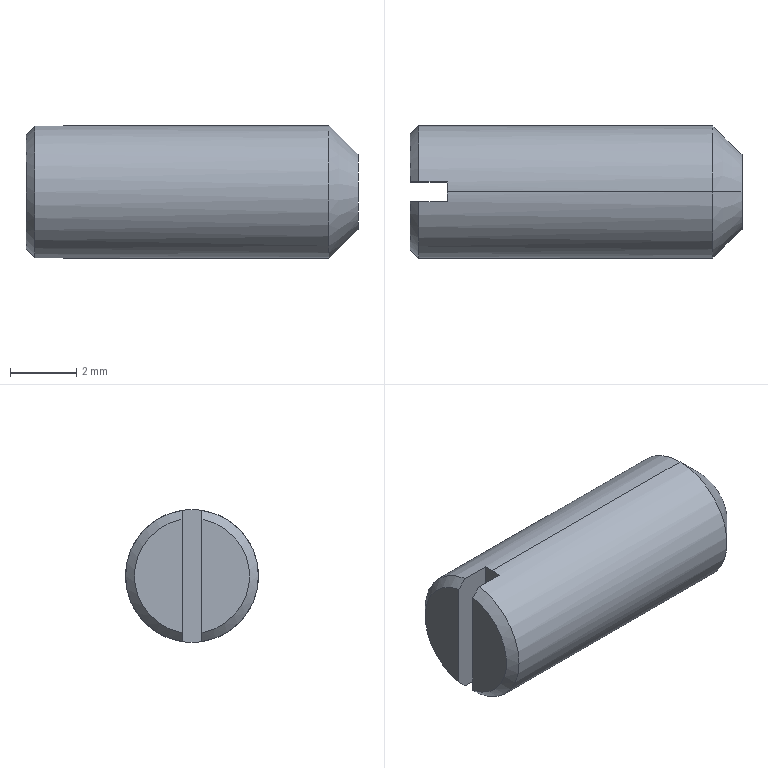Part | STEP file | 1 solid | 12 faces | box 10 x 4 x 4 mm | volume 118.489 mm3 | plane 6 | cone 4 | cylinder 2 | commonest cylinder face diameters 4 x2
STEP:
#1=CARTESIAN_POINT('',(0.,0.,0.));
#2=DIRECTION('',(0.,0.,1.));
#3=DIRECTION('',(1.,0.,0.));
#4=AXIS2_PLACEMENT_3D('',#1,#2,#3);
#5=CARTESIAN_POINT('',(1.12,-0.3,-1.977));
#6=VERTEX_POINT('',#5);
#7=CARTESIAN_POINT('',(1.12,0.,-2.));
#8=VERTEX_POINT('',#7);
#9=CARTESIAN_POINT('',(1.12,0.,0.));
#10=DIRECTION('',(1.,0.,0.));
#11=DIRECTION('',(0.,0.,1.));
#12=AXIS2_PLACEMENT_3D('',#9,#10,#11);
#13=CIRCLE('',#12,2.);
#14=CARTESIAN_POINT('',(1.12,-0.3,-50.));
#15=DIRECTION('',(1.,0.,0.));
#16=DIRECTION('',(0.,1.,0.));
#17=AXIS2_PLACEMENT_3D('',#14,#15,#16);
#18=PLANE('',#17);
#19=CARTESIAN_POINT('',(0.3,50.));
#20=DIRECTION('',(0.,1.));
#21=AXIS2_PLACEMENT_2D('',#19,#20);
#22=CIRCLE('',#21,2.);
#23=(GEOMETRIC_REPRESENTATION_CONTEXT(2)PARAMETRIC_REPRESENTATION_CONTEXT()REPRESENTATION_CONTEXT('',''));
#24=DEFINITIONAL_REPRESENTATION('',(#22),#23);
#25=PCURVE('',#18,#24);
#26=CARTESIAN_POINT('',(-0.5499,0.,0.));
#27=DIRECTION('',(-1.,0.,0.));
#28=DIRECTION('',(0.,0.,1.));
#29=AXIS2_PLACEMENT_3D('',#26,#27,#28);
#30=CYLINDRICAL_SURFACE('',#29,2.);
#31=CARTESIAN_POINT('',(6.283,-1.67));
#32=DIRECTION('',(-1.,0.));
#33=VECTOR('',#32,1.);
#34=LINE('',#31,#33);
#35=(GEOMETRIC_REPRESENTATION_CONTEXT(2)PARAMETRIC_REPRESENTATION_CONTEXT()REPRESENTATION_CONTEXT('',''));
#36=DEFINITIONAL_REPRESENTATION('',(#34),#35);
#37=PCURVE('',#30,#36);
#38=SURFACE_CURVE('',#13,(#25,#37),.PCURVE_S1.);
#39=EDGE_CURVE('',#6,#8,#38,.T.);
#40=ORIENTED_EDGE('',*,*,#39,.F.);
#41=CARTESIAN_POINT('',(1.12,-0.3,1.977));
#42=VERTEX_POINT('',#41);
#43=CARTESIAN_POINT('',(1.12,-0.3,-50.));
#44=DIRECTION('',(0.,0.,1.));
#45=VECTOR('',#44,1.);
#46=LINE('',#43,#45);
#47=CARTESIAN_POINT('',(0.,0.));
#48=DIRECTION('',(0.,1.));
#49=VECTOR('',#48,1.);
#50=LINE('',#47,#49);
#51=(GEOMETRIC_REPRESENTATION_CONTEXT(2)PARAMETRIC_REPRESENTATION_CONTEXT()REPRESENTATION_CONTEXT('',''));
#52=DEFINITIONAL_REPRESENTATION('',(#50),#51);
#53=PCURVE('',#18,#52);
#54=CARTESIAN_POINT('',(0.,-0.3,-50.));
#55=DIRECTION('',(0.,-1.,0.));
#56=DIRECTION('',(0.,0.,-1.));
#57=AXIS2_PLACEMENT_3D('',#54,#55,#56);
#58=PLANE('',#57);
#59=CARTESIAN_POINT('',(0.,1.12));
#60=DIRECTION('',(-1.,0.));
#61=VECTOR('',#60,1.);
#62=LINE('',#59,#61);
#63=(GEOMETRIC_REPRESENTATION_CONTEXT(2)PARAMETRIC_REPRESENTATION_CONTEXT()REPRESENTATION_CONTEXT('',''));
#64=DEFINITIONAL_REPRESENTATION('',(#62),#63);
#65=PCURVE('',#58,#64);
#66=SURFACE_CURVE('',#46,(#53,#65),.PCURVE_S1.);
#67=EDGE_CURVE('',#6,#42,#66,.T.);
#68=ORIENTED_EDGE('',*,*,#67,.T.);
#69=CARTESIAN_POINT('',(1.12,0.,2.));
#70=VERTEX_POINT('',#69);
#71=CARTESIAN_POINT('',(1.12,0.,0.));
#72=DIRECTION('',(1.,0.,0.));
#73=DIRECTION('',(0.,0.,1.));
#74=AXIS2_PLACEMENT_3D('',#71,#72,#73);
#75=CIRCLE('',#74,2.);
#76=CARTESIAN_POINT('',(0.3,50.));
#77=DIRECTION('',(0.,1.));
#78=AXIS2_PLACEMENT_2D('',#76,#77);
#79=CIRCLE('',#78,2.);
#80=(GEOMETRIC_REPRESENTATION_CONTEXT(2)PARAMETRIC_REPRESENTATION_CONTEXT()REPRESENTATION_CONTEXT('',''));
#81=DEFINITIONAL_REPRESENTATION('',(#79),#80);
#82=PCURVE('',#18,#81);
#83=CARTESIAN_POINT('',(6.283,-1.67));
#84=DIRECTION('',(-1.,0.));
#85=VECTOR('',#84,1.);
#86=LINE('',#83,#85);
#87=(GEOMETRIC_REPRESENTATION_CONTEXT(2)PARAMETRIC_REPRESENTATION_CONTEXT()REPRESENTATION_CONTEXT('',''));
#88=DEFINITIONAL_REPRESENTATION('',(#86),#87);
#89=PCURVE('',#30,#88);
#90=SURFACE_CURVE('',#75,(#82,#89),.PCURVE_S1.);
#91=EDGE_CURVE('',#70,#42,#90,.T.);
#92=ORIENTED_EDGE('',*,*,#91,.F.);
#93=CARTESIAN_POINT('',(1.12,0.3,1.977));
#94=VERTEX_POINT('',#93);
#95=CARTESIAN_POINT('',(1.12,0.,0.));
#96=DIRECTION('',(1.,0.,0.));
#97=DIRECTION('',(0.,0.,1.));
#98=AXIS2_PLACEMENT_3D('',#95,#96,#97);
#99=CIRCLE('',#98,2.);
#100=CARTESIAN_POINT('',(0.3,50.));
#101=DIRECTION('',(0.,1.));
#102=AXIS2_PLACEMENT_2D('',#100,#101);
#103=CIRCLE('',#102,2.);
#104=(GEOMETRIC_REPRESENTATION_CONTEXT(2)PARAMETRIC_REPRESENTATION_CONTEXT()REPRESENTATION_CONTEXT('',''));
#105=DEFINITIONAL_REPRESENTATION('',(#103),#104);
#106=PCURVE('',#18,#105);
#107=CARTESIAN_POINT('',(-0.5499,0.,0.));
#108=DIRECTION('',(-1.,0.,0.));
#109=DIRECTION('',(0.,0.,1.));
#110=AXIS2_PLACEMENT_3D('',#107,#108,#109);
#111=CYLINDRICAL_SURFACE('',#110,2.);
#112=CARTESIAN_POINT('',(6.283,-1.67));
#113=DIRECTION('',(-1.,0.));
#114=VECTOR('',#113,1.);
#115=LINE('',#112,#114);
#116=(GEOMETRIC_REPRESENTATION_CONTEXT(2)PARAMETRIC_REPRESENTATION_CONTEXT()REPRESENTATION_CONTEXT('',''));
#117=DEFINITIONAL_REPRESENTATION('',(#115),#116);
#118=PCURVE('',#111,#117);
#119=SURFACE_CURVE('',#99,(#106,#118),.PCURVE_S1.);
#120=EDGE_CURVE('',#94,#70,#119,.T.);
#121=ORIENTED_EDGE('',*,*,#120,.F.);
#122=CARTESIAN_POINT('',(1.12,0.3,-1.977));
#123=VERTEX_POINT('',#122);
#124=CARTESIAN_POINT('',(1.12,0.3,-50.));
#125=DIRECTION('',(0.,0.,-1.));
#126=VECTOR('',#125,1.);
#127=LINE('',#124,#126);
#128=CARTESIAN_POINT('',(0.6,0.));
#129=DIRECTION('',(0.,-1.));
#130=VECTOR('',#129,1.);
#131=LINE('',#128,#130);
#132=(GEOMETRIC_REPRESENTATION_CONTEXT(2)PARAMETRIC_REPRESENTATION_CONTEXT()REPRESENTATION_CONTEXT('',''));
#133=DEFINITIONAL_REPRESENTATION('',(#131),#132);
#134=PCURVE('',#18,#133);
#135=CARTESIAN_POINT('',(0.,0.3,-50.));
#136=DIRECTION('',(0.,1.,0.));
#137=DIRECTION('',(1.,0.,0.));
#138=AXIS2_PLACEMENT_3D('',#135,#136,#137);
#139=PLANE('',#138);
#140=CARTESIAN_POINT('',(1.12,0.));
#141=DIRECTION('',(0.,1.));
#142=VECTOR('',#141,1.);
#143=LINE('',#140,#142);
#144=(GEOMETRIC_REPRESENTATION_CONTEXT(2)PARAMETRIC_REPRESENTATION_CONTEXT()REPRESENTATION_CONTEXT('',''));
#145=DEFINITIONAL_REPRESENTATION('',(#143),#144);
#146=PCURVE('',#139,#145);
#147=SURFACE_CURVE('',#127,(#134,#146),.PCURVE_S1.);
#148=EDGE_CURVE('',#94,#123,#147,.T.);
#149=ORIENTED_EDGE('',*,*,#148,.T.);
#150=CARTESIAN_POINT('',(1.12,0.,0.));
#151=DIRECTION('',(1.,0.,0.));
#152=DIRECTION('',(0.,0.,1.));
#153=AXIS2_PLACEMENT_3D('',#150,#151,#152);
#154=CIRCLE('',#153,2.);
#155=CARTESIAN_POINT('',(0.3,50.));
#156=DIRECTION('',(0.,1.));
#157=AXIS2_PLACEMENT_2D('',#155,#156);
#158=CIRCLE('',#157,2.);
#159=(GEOMETRIC_REPRESENTATION_CONTEXT(2)PARAMETRIC_REPRESENTATION_CONTEXT()REPRESENTATION_CONTEXT('',''));
#160=DEFINITIONAL_REPRESENTATION('',(#158),#159);
#161=PCURVE('',#18,#160);
#162=CARTESIAN_POINT('',(6.283,-1.67));
#163=DIRECTION('',(-1.,0.));
#164=VECTOR('',#163,1.);
#165=LINE('',#162,#164);
#166=(GEOMETRIC_REPRESENTATION_CONTEXT(2)PARAMETRIC_REPRESENTATION_CONTEXT()REPRESENTATION_CONTEXT('',''));
#167=DEFINITIONAL_REPRESENTATION('',(#165),#166);
#168=PCURVE('',#111,#167);
#169=SURFACE_CURVE('',#154,(#161,#168),.PCURVE_S1.);
#170=EDGE_CURVE('',#8,#123,#169,.T.);
#171=ORIENTED_EDGE('',*,*,#170,.F.);
#172=EDGE_LOOP('',(#40,#68,#92,#121,#149,#171));
#173=FACE_BOUND('',#172,.T.);
#174=ADVANCED_FACE('',(#173),#18,.F.);
#175=CARTESIAN_POINT('',(0.268,-0.3,-1.977));
#176=VERTEX_POINT('',#175);
#177=CARTESIAN_POINT('',(0.,-0.3,-1.977));
#178=DIRECTION('',(1.,0.,0.));
#179=VECTOR('',#178,1.);
#180=LINE('',#177,#179);
#181=CARTESIAN_POINT('',(-48.023,0.));
#182=DIRECTION('',(0.,1.));
#183=VECTOR('',#182,1.);
#184=LINE('',#181,#183);
#185=(GEOMETRIC_REPRESENTATION_CONTEXT(2)PARAMETRIC_REPRESENTATION_CONTEXT()REPRESENTATION_CONTEXT('',''));
#186=DEFINITIONAL_REPRESENTATION('',(#184),#185);
#187=PCURVE('',#58,#186);
#188=CARTESIAN_POINT('',(3.292,-0.5499));
#189=DIRECTION('',(0.,-1.));
#190=VECTOR('',#189,1.);
#191=LINE('',#188,#190);
#192=(GEOMETRIC_REPRESENTATION_CONTEXT(2)PARAMETRIC_REPRESENTATION_CONTEXT()REPRESENTATION_CONTEXT('',''));
#193=DEFINITIONAL_REPRESENTATION('',(#191),#192);
#194=PCURVE('',#30,#193);
#195=SURFACE_CURVE('',#180,(#187,#194),.PCURVE_S1.);
#196=EDGE_CURVE('',#176,#6,#195,.T.);
#197=ORIENTED_EDGE('',*,*,#196,.F.);
#198=CARTESIAN_POINT('',(0.,-0.3,-1.706));
#199=VERTEX_POINT('',#198);
#200=CARTESIAN_POINT('',(0.,-0.3,-1.706));
#201=CARTESIAN_POINT('',(0.08924,-0.3,-1.796));
#202=CARTESIAN_POINT('',(0.1786,-0.3,-1.887));
#203=CARTESIAN_POINT('',(0.268,-0.3,-1.977));
#204=B_SPLINE_CURVE_WITH_KNOTS('',3,(#200,#201,#202,#203),.UNSPECIFIED.,.F.,.F.,(4,4),(0.,0.0003815),.PIECEWISE_BEZIER_KNOTS.);
#205=CARTESIAN_POINT('',(-48.294,0.));
#206=CARTESIAN_POINT('',(-48.204,0.08924));
#207=CARTESIAN_POINT('',(-48.113,0.1786));
#208=CARTESIAN_POINT('',(-48.023,0.268));
#209=B_SPLINE_CURVE_WITH_KNOTS('',3,(#205,#206,#207,#208),.UNSPECIFIED.,.F.,.F.,(4,4),(0.,0.0003815),.PIECEWISE_BEZIER_KNOTS.);
#210=(GEOMETRIC_REPRESENTATION_CONTEXT(2)PARAMETRIC_REPRESENTATION_CONTEXT()REPRESENTATION_CONTEXT('',''));
#211=DEFINITIONAL_REPRESENTATION('',(#209),#210);
#212=PCURVE('',#58,#211);
#213=CARTESIAN_POINT('',(0.268,0.,0.));
#214=DIRECTION('',(1.,0.,0.));
#215=DIRECTION('',(0.,0.,-1.));
#216=AXIS2_PLACEMENT_3D('',#213,#214,#215);
#217=CONICAL_SURFACE('',#216,2.,0.7854);
#218=CARTESIAN_POINT('',(6.109,-0.268));
#219=CARTESIAN_POINT('',(6.11,-0.2639));
#220=CARTESIAN_POINT('',(6.11,-0.2558));
#221=CARTESIAN_POINT('',(6.112,-0.2437));
#222=CARTESIAN_POINT('',(6.113,-0.2315));
#223=CARTESIAN_POINT('',(6.114,-0.2193));
#224=CARTESIAN_POINT('',(6.115,-0.2071));
#225=CARTESIAN_POINT('',(6.116,-0.195));
#226=CARTESIAN_POINT('',(6.117,-0.1828));
#227=CARTESIAN_POINT('',(6.118,-0.1706));
#228=CARTESIAN_POINT('',(6.12,-0.1584));
#229=CARTESIAN_POINT('',(6.121,-0.1462));
#230=CARTESIAN_POINT('',(6.122,-0.1341));
#231=CARTESIAN_POINT('',(6.123,-0.1219));
#232=CARTESIAN_POINT('',(6.124,-0.1097));
#233=CARTESIAN_POINT('',(6.125,-0.09751));
#234=CARTESIAN_POINT('',(6.126,-0.08533));
#235=CARTESIAN_POINT('',(6.127,-0.07314));
#236=CARTESIAN_POINT('',(6.128,-0.06095));
#237=CARTESIAN_POINT('',(6.129,-0.04876));
#238=CARTESIAN_POINT('',(6.13,-0.03657));
#239=CARTESIAN_POINT('',(6.131,-0.02438));
#240=CARTESIAN_POINT('',(6.132,-0.01219));
#241=CARTESIAN_POINT('',(6.132,-0.004064));
#242=CARTESIAN_POINT('',(6.133,0.));
#243=B_SPLINE_CURVE_WITH_KNOTS('',3,(#218,#219,#220,#221,#222,#223,#224,#225,#226,#227,#228,#229,#230,#231,#232,#233,#234,#235,#236,#237,#238,#239,#240,#241,#242),.UNSPECIFIED.,.F.,.F.,(4,1,1,1,1,1,1,1,1,1,1,1,1,1,1,1,1,1,1,1,1,1,4),(0.,0.00001734,0.00003468,0.00005203,0.00006937,0.00008671,0.0001041,0.0001214,0.0001387,0.0001561,0.0001734,0.0001908,0.0002081,0.0002254,0.0002428,0.0002601,0.0002775,0.0002948,0.0003122,0.0003295,0.0003468,0.0003642,0.0003815),.QUASI_UNIFORM_KNOTS.);
#244=(GEOMETRIC_REPRESENTATION_CONTEXT(2)PARAMETRIC_REPRESENTATION_CONTEXT()REPRESENTATION_CONTEXT('',''));
#245=DEFINITIONAL_REPRESENTATION('',(#243),#244);
#246=PCURVE('',#217,#245);
#247=SURFACE_CURVE('',#204,(#212,#246),.PCURVE_S1.);
#248=EDGE_CURVE('',#199,#176,#247,.T.);
#249=ORIENTED_EDGE('',*,*,#248,.F.);
#250=CARTESIAN_POINT('',(0.,-0.3,1.706));
#251=VERTEX_POINT('',#250);
#252=CARTESIAN_POINT('',(0.,-0.3,0.));
#253=DIRECTION('',(0.,0.,1.));
#254=VECTOR('',#253,1.);
#255=LINE('',#252,#254);
#256=CARTESIAN_POINT('',(-50.,0.));
#257=DIRECTION('',(-1.,0.));
#258=VECTOR('',#257,1.);
#259=LINE('',#256,#258);
#260=(GEOMETRIC_REPRESENTATION_CONTEXT(2)PARAMETRIC_REPRESENTATION_CONTEXT()REPRESENTATION_CONTEXT('',''));
#261=DEFINITIONAL_REPRESENTATION('',(#259),#260);
#262=PCURVE('',#58,#261);
#263=CARTESIAN_POINT('',(0.,1.732,0.));
#264=DIRECTION('',(1.,0.,0.));
#265=DIRECTION('',(0.,1.,0.));
#266=AXIS2_PLACEMENT_3D('',#263,#264,#265);
#267=PLANE('',#266);
#268=CARTESIAN_POINT('',(-2.032,0.));
#269=DIRECTION('',(0.,1.));
#270=VECTOR('',#269,1.);
#271=LINE('',#268,#270);
#272=(GEOMETRIC_REPRESENTATION_CONTEXT(2)PARAMETRIC_REPRESENTATION_CONTEXT()REPRESENTATION_CONTEXT('',''));
#273=DEFINITIONAL_REPRESENTATION('',(#271),#272);
#274=PCURVE('',#267,#273);
#275=SURFACE_CURVE('',#255,(#262,#274),.PCURVE_S1.);
#276=EDGE_CURVE('',#199,#251,#275,.T.);
#277=ORIENTED_EDGE('',*,*,#276,.T.);
#278=CARTESIAN_POINT('',(0.268,-0.3,1.977));
#279=VERTEX_POINT('',#278);
#280=CARTESIAN_POINT('',(0.268,-0.3,1.977));
#281=CARTESIAN_POINT('',(0.1786,-0.3,1.887));
#282=CARTESIAN_POINT('',(0.08924,-0.3,1.796));
#283=CARTESIAN_POINT('',(0.,-0.3,1.706));
#284=B_SPLINE_CURVE_WITH_KNOTS('',3,(#280,#281,#282,#283),.UNSPECIFIED.,.F.,.F.,(4,4),(0.,0.0003815),.PIECEWISE_BEZIER_KNOTS.);
#285=CARTESIAN_POINT('',(-51.977,0.268));
#286=CARTESIAN_POINT('',(-51.887,0.1786));
#287=CARTESIAN_POINT('',(-51.796,0.08924));
#288=CARTESIAN_POINT('',(-51.706,0.));
#289=B_SPLINE_CURVE_WITH_KNOTS('',3,(#285,#286,#287,#288),.UNSPECIFIED.,.F.,.F.,(4,4),(0.,0.0003815),.PIECEWISE_BEZIER_KNOTS.);
#290=(GEOMETRIC_REPRESENTATION_CONTEXT(2)PARAMETRIC_REPRESENTATION_CONTEXT()REPRESENTATION_CONTEXT('',''));
#291=DEFINITIONAL_REPRESENTATION('',(#289),#290);
#292=PCURVE('',#58,#291);
#293=CARTESIAN_POINT('',(3.292,0.));
#294=CARTESIAN_POINT('',(3.292,-0.004064));
#295=CARTESIAN_POINT('',(3.293,-0.01219));
#296=CARTESIAN_POINT('',(3.294,-0.02438));
#297=CARTESIAN_POINT('',(3.295,-0.03657));
#298=CARTESIAN_POINT('',(3.296,-0.04876));
#299=CARTESIAN_POINT('',(3.297,-0.06095));
#300=CARTESIAN_POINT('',(3.298,-0.07314));
#301=CARTESIAN_POINT('',(3.299,-0.08533));
#302=CARTESIAN_POINT('',(3.3,-0.09751));
#303=CARTESIAN_POINT('',(3.301,-0.1097));
#304=CARTESIAN_POINT('',(3.302,-0.1219));
#305=CARTESIAN_POINT('',(3.303,-0.1341));
#306=CARTESIAN_POINT('',(3.304,-0.1462));
#307=CARTESIAN_POINT('',(3.305,-0.1584));
#308=CARTESIAN_POINT('',(3.306,-0.1706));
#309=CARTESIAN_POINT('',(3.307,-0.1828));
#310=CARTESIAN_POINT('',(3.309,-0.195));
#311=CARTESIAN_POINT('',(3.31,-0.2071));
#312=CARTESIAN_POINT('',(3.311,-0.2193));
#313=CARTESIAN_POINT('',(3.312,-0.2315));
#314=CARTESIAN_POINT('',(3.313,-0.2437));
#315=CARTESIAN_POINT('',(3.314,-0.2558));
#316=CARTESIAN_POINT('',(3.315,-0.2639));
#317=CARTESIAN_POINT('',(3.316,-0.268));
#318=B_SPLINE_CURVE_WITH_KNOTS('',3,(#293,#294,#295,#296,#297,#298,#299,#300,#301,#302,#303,#304,#305,#306,#307,#308,#309,#310,#311,#312,#313,#314,#315,#316,#317),.UNSPECIFIED.,.F.,.F.,(4,1,1,1,1,1,1,1,1,1,1,1,1,1,1,1,1,1,1,1,1,1,4),(0.,0.00001734,0.00003468,0.00005203,0.00006937,0.00008671,0.0001041,0.0001214,0.0001387,0.0001561,0.0001734,0.0001908,0.0002081,0.0002254,0.0002428,0.0002601,0.0002775,0.0002948,0.0003122,0.0003295,0.0003468,0.0003642,0.0003815),.QUASI_UNIFORM_KNOTS.);
#319=(GEOMETRIC_REPRESENTATION_CONTEXT(2)PARAMETRIC_REPRESENTATION_CONTEXT()REPRESENTATION_CONTEXT('',''));
#320=DEFINITIONAL_REPRESENTATION('',(#318),#319);
#321=PCURVE('',#217,#320);
#322=SURFACE_CURVE('',#284,(#292,#321),.PCURVE_S1.);
#323=EDGE_CURVE('',#279,#251,#322,.T.);
#324=ORIENTED_EDGE('',*,*,#323,.F.);
#325=CARTESIAN_POINT('',(0.,-0.3,1.977));
#326=DIRECTION('',(-1.,0.,0.));
#327=VECTOR('',#326,1.);
#328=LINE('',#325,#327);
#329=CARTESIAN_POINT('',(-51.977,0.));
#330=DIRECTION('',(0.,-1.));
#331=VECTOR('',#330,1.);
#332=LINE('',#329,#331);
#333=(GEOMETRIC_REPRESENTATION_CONTEXT(2)PARAMETRIC_REPRESENTATION_CONTEXT()REPRESENTATION_CONTEXT('',''));
#334=DEFINITIONAL_REPRESENTATION('',(#332),#333);
#335=PCURVE('',#58,#334);
#336=CARTESIAN_POINT('',(6.133,-0.5499));
#337=DIRECTION('',(0.,1.));
#338=VECTOR('',#337,1.);
#339=LINE('',#336,#338);
#340=(GEOMETRIC_REPRESENTATION_CONTEXT(2)PARAMETRIC_REPRESENTATION_CONTEXT()REPRESENTATION_CONTEXT('',''));
#341=DEFINITIONAL_REPRESENTATION('',(#339),#340);
#342=PCURVE('',#30,#341);
#343=SURFACE_CURVE('',#328,(#335,#342),.PCURVE_S1.);
#344=EDGE_CURVE('',#42,#279,#343,.T.);
#345=ORIENTED_EDGE('',*,*,#344,.F.);
#346=ORIENTED_EDGE('',*,*,#67,.F.);
#347=EDGE_LOOP('',(#197,#249,#277,#324,#345,#346));
#348=FACE_BOUND('',#347,.T.);
#349=ADVANCED_FACE('',(#348),#58,.F.);
#350=CARTESIAN_POINT('',(0.268,0.3,1.977));
#351=VERTEX_POINT('',#350);
#352=CARTESIAN_POINT('',(0.,0.3,1.977));
#353=DIRECTION('',(1.,0.,0.));
#354=VECTOR('',#353,1.);
#355=LINE('',#352,#354);
#356=CARTESIAN_POINT('',(0.,-51.977));
#357=DIRECTION('',(1.,0.));
#358=VECTOR('',#357,1.);
#359=LINE('',#356,#358);
#360=(GEOMETRIC_REPRESENTATION_CONTEXT(2)PARAMETRIC_REPRESENTATION_CONTEXT()REPRESENTATION_CONTEXT('',''));
#361=DEFINITIONAL_REPRESENTATION('',(#359),#360);
#362=PCURVE('',#139,#361);
#363=CARTESIAN_POINT('',(0.1506,-0.5499));
#364=DIRECTION('',(0.,-1.));
#365=VECTOR('',#364,1.);
#366=LINE('',#363,#365);
#367=(GEOMETRIC_REPRESENTATION_CONTEXT(2)PARAMETRIC_REPRESENTATION_CONTEXT()REPRESENTATION_CONTEXT('',''));
#368=DEFINITIONAL_REPRESENTATION('',(#366),#367);
#369=PCURVE('',#111,#368);
#370=SURFACE_CURVE('',#355,(#362,#369),.PCURVE_S1.);
#371=EDGE_CURVE('',#351,#94,#370,.T.);
#372=ORIENTED_EDGE('',*,*,#371,.F.);
#373=CARTESIAN_POINT('',(0.,0.3,1.706));
#374=VERTEX_POINT('',#373);
#375=CARTESIAN_POINT('',(0.,0.3,1.706));
#376=CARTESIAN_POINT('',(0.08924,0.3,1.796));
#377=CARTESIAN_POINT('',(0.1786,0.3,1.887));
#378=CARTESIAN_POINT('',(0.268,0.3,1.977));
#379=B_SPLINE_CURVE_WITH_KNOTS('',3,(#375,#376,#377,#378),.UNSPECIFIED.,.F.,.F.,(4,4),(0.,0.0003815),.PIECEWISE_BEZIER_KNOTS.);
#380=CARTESIAN_POINT('',(0.,-51.706));
#381=CARTESIAN_POINT('',(0.08924,-51.796));
#382=CARTESIAN_POINT('',(0.1786,-51.887));
#383=CARTESIAN_POINT('',(0.268,-51.977));
#384=B_SPLINE_CURVE_WITH_KNOTS('',3,(#380,#381,#382,#383),.UNSPECIFIED.,.F.,.F.,(4,4),(0.,0.0003815),.PIECEWISE_BEZIER_KNOTS.);
#385=(GEOMETRIC_REPRESENTATION_CONTEXT(2)PARAMETRIC_REPRESENTATION_CONTEXT()REPRESENTATION_CONTEXT('',''));
#386=DEFINITIONAL_REPRESENTATION('',(#384),#385);
#387=PCURVE('',#139,#386);
#388=CARTESIAN_POINT('',(0.268,0.,0.));
#389=DIRECTION('',(1.,0.,0.));
#390=DIRECTION('',(0.,0.,-1.));
#391=AXIS2_PLACEMENT_3D('',#388,#389,#390);
#392=CONICAL_SURFACE('',#391,2.,0.7854);
#393=CARTESIAN_POINT('',(2.968,-0.268));
#394=CARTESIAN_POINT('',(2.968,-0.2639));
#395=CARTESIAN_POINT('',(2.969,-0.2558));
#396=CARTESIAN_POINT('',(2.97,-0.2437));
#397=CARTESIAN_POINT('',(2.971,-0.2315));
#398=CARTESIAN_POINT('',(2.972,-0.2193));
#399=CARTESIAN_POINT('',(2.973,-0.2071));
#400=CARTESIAN_POINT('',(2.975,-0.195));
#401=CARTESIAN_POINT('',(2.976,-0.1828));
#402=CARTESIAN_POINT('',(2.977,-0.1706));
#403=CARTESIAN_POINT('',(2.978,-0.1584));
#404=CARTESIAN_POINT('',(2.979,-0.1462));
#405=CARTESIAN_POINT('',(2.98,-0.1341));
#406=CARTESIAN_POINT('',(2.981,-0.1219));
#407=CARTESIAN_POINT('',(2.982,-0.1097));
#408=CARTESIAN_POINT('',(2.983,-0.09751));
#409=CARTESIAN_POINT('',(2.984,-0.08533));
#410=CARTESIAN_POINT('',(2.985,-0.07314));
#411=CARTESIAN_POINT('',(2.986,-0.06095));
#412=CARTESIAN_POINT('',(2.987,-0.04876));
#413=CARTESIAN_POINT('',(2.988,-0.03657));
#414=CARTESIAN_POINT('',(2.989,-0.02438));
#415=CARTESIAN_POINT('',(2.99,-0.01219));
#416=CARTESIAN_POINT('',(2.991,-0.004064));
#417=CARTESIAN_POINT('',(2.991,0.));
#418=B_SPLINE_CURVE_WITH_KNOTS('',3,(#393,#394,#395,#396,#397,#398,#399,#400,#401,#402,#403,#404,#405,#406,#407,#408,#409,#410,#411,#412,#413,#414,#415,#416,#417),.UNSPECIFIED.,.F.,.F.,(4,1,1,1,1,1,1,1,1,1,1,1,1,1,1,1,1,1,1,1,1,1,4),(0.,0.00001734,0.00003468,0.00005203,0.00006937,0.00008671,0.0001041,0.0001214,0.0001387,0.0001561,0.0001734,0.0001908,0.0002081,0.0002254,0.0002428,0.0002601,0.0002775,0.0002948,0.0003122,0.0003295,0.0003468,0.0003642,0.0003815),.QUASI_UNIFORM_KNOTS.);
#419=(GEOMETRIC_REPRESENTATION_CONTEXT(2)PARAMETRIC_REPRESENTATION_CONTEXT()REPRESENTATION_CONTEXT('',''));
#420=DEFINITIONAL_REPRESENTATION('',(#418),#419);
#421=PCURVE('',#392,#420);
#422=SURFACE_CURVE('',#379,(#387,#421),.PCURVE_S1.);
#423=EDGE_CURVE('',#374,#351,#422,.T.);
#424=ORIENTED_EDGE('',*,*,#423,.F.);
#425=CARTESIAN_POINT('',(0.,0.3,-1.706));
#426=VERTEX_POINT('',#425);
#427=CARTESIAN_POINT('',(0.,0.3,0.));
#428=DIRECTION('',(0.,0.,-1.));
#429=VECTOR('',#428,1.);
#430=LINE('',#427,#429);
#431=CARTESIAN_POINT('',(0.,-50.));
#432=DIRECTION('',(0.,1.));
#433=VECTOR('',#432,1.);
#434=LINE('',#431,#433);
#435=(GEOMETRIC_REPRESENTATION_CONTEXT(2)PARAMETRIC_REPRESENTATION_CONTEXT()REPRESENTATION_CONTEXT('',''));
#436=DEFINITIONAL_REPRESENTATION('',(#434),#435);
#437=PCURVE('',#139,#436);
#438=CARTESIAN_POINT('',(0.,1.732,0.));
#439=DIRECTION('',(1.,0.,0.));
#440=DIRECTION('',(0.,1.,0.));
#441=AXIS2_PLACEMENT_3D('',#438,#439,#440);
#442=PLANE('',#441);
#443=CARTESIAN_POINT('',(-1.432,0.));
#444=DIRECTION('',(0.,-1.));
#445=VECTOR('',#444,1.);
#446=LINE('',#443,#445);
#447=(GEOMETRIC_REPRESENTATION_CONTEXT(2)PARAMETRIC_REPRESENTATION_CONTEXT()REPRESENTATION_CONTEXT('',''));
#448=DEFINITIONAL_REPRESENTATION('',(#446),#447);
#449=PCURVE('',#442,#448);
#450=SURFACE_CURVE('',#430,(#437,#449),.PCURVE_S1.);
#451=EDGE_CURVE('',#374,#426,#450,.T.);
#452=ORIENTED_EDGE('',*,*,#451,.T.);
#453=CARTESIAN_POINT('',(0.268,0.3,-1.977));
#454=VERTEX_POINT('',#453);
#455=CARTESIAN_POINT('',(0.268,0.3,-1.977));
#456=CARTESIAN_POINT('',(0.1786,0.3,-1.887));
#457=CARTESIAN_POINT('',(0.08924,0.3,-1.796));
#458=CARTESIAN_POINT('',(0.,0.3,-1.706));
#459=B_SPLINE_CURVE_WITH_KNOTS('',3,(#455,#456,#457,#458),.UNSPECIFIED.,.F.,.F.,(4,4),(0.,0.0003815),.PIECEWISE_BEZIER_KNOTS.);
#460=CARTESIAN_POINT('',(0.268,-48.023));
#461=CARTESIAN_POINT('',(0.1786,-48.113));
#462=CARTESIAN_POINT('',(0.08924,-48.204));
#463=CARTESIAN_POINT('',(0.,-48.294));
#464=B_SPLINE_CURVE_WITH_KNOTS('',3,(#460,#461,#462,#463),.UNSPECIFIED.,.F.,.F.,(4,4),(0.,0.0003815),.PIECEWISE_BEZIER_KNOTS.);
#465=(GEOMETRIC_REPRESENTATION_CONTEXT(2)PARAMETRIC_REPRESENTATION_CONTEXT()REPRESENTATION_CONTEXT('',''));
#466=DEFINITIONAL_REPRESENTATION('',(#464),#465);
#467=PCURVE('',#139,#466);
#468=CARTESIAN_POINT('',(0.1506,0.));
#469=CARTESIAN_POINT('',(0.1509,-0.004064));
#470=CARTESIAN_POINT('',(0.1515,-0.01219));
#471=CARTESIAN_POINT('',(0.1524,-0.02438));
#472=CARTESIAN_POINT('',(0.1534,-0.03657));
#473=CARTESIAN_POINT('',(0.1544,-0.04876));
#474=CARTESIAN_POINT('',(0.1553,-0.06095));
#475=CARTESIAN_POINT('',(0.1563,-0.07314));
#476=CARTESIAN_POINT('',(0.1573,-0.08533));
#477=CARTESIAN_POINT('',(0.1583,-0.09751));
#478=CARTESIAN_POINT('',(0.1594,-0.1097));
#479=CARTESIAN_POINT('',(0.1604,-0.1219));
#480=CARTESIAN_POINT('',(0.1615,-0.1341));
#481=CARTESIAN_POINT('',(0.1625,-0.1462));
#482=CARTESIAN_POINT('',(0.1636,-0.1584));
#483=CARTESIAN_POINT('',(0.1647,-0.1706));
#484=CARTESIAN_POINT('',(0.1658,-0.1828));
#485=CARTESIAN_POINT('',(0.167,-0.195));
#486=CARTESIAN_POINT('',(0.1681,-0.2071));
#487=CARTESIAN_POINT('',(0.1693,-0.2193));
#488=CARTESIAN_POINT('',(0.1705,-0.2315));
#489=CARTESIAN_POINT('',(0.1716,-0.2437));
#490=CARTESIAN_POINT('',(0.1729,-0.2558));
#491=CARTESIAN_POINT('',(0.1737,-0.2639));
#492=CARTESIAN_POINT('',(0.1741,-0.268));
#493=B_SPLINE_CURVE_WITH_KNOTS('',3,(#468,#469,#470,#471,#472,#473,#474,#475,#476,#477,#478,#479,#480,#481,#482,#483,#484,#485,#486,#487,#488,#489,#490,#491,#492),.UNSPECIFIED.,.F.,.F.,(4,1,1,1,1,1,1,1,1,1,1,1,1,1,1,1,1,1,1,1,1,1,4),(0.,0.00001734,0.00003468,0.00005203,0.00006937,0.00008671,0.0001041,0.0001214,0.0001387,0.0001561,0.0001734,0.0001908,0.0002081,0.0002254,0.0002428,0.0002601,0.0002775,0.0002948,0.0003122,0.0003295,0.0003468,0.0003642,0.0003815),.QUASI_UNIFORM_KNOTS.);
#494=(GEOMETRIC_REPRESENTATION_CONTEXT(2)PARAMETRIC_REPRESENTATION_CONTEXT()REPRESENTATION_CONTEXT('',''));
#495=DEFINITIONAL_REPRESENTATION('',(#493),#494);
#496=PCURVE('',#392,#495);
#497=SURFACE_CURVE('',#459,(#467,#496),.PCURVE_S1.);
#498=EDGE_CURVE('',#454,#426,#497,.T.);
#499=ORIENTED_EDGE('',*,*,#498,.F.);
#500=CARTESIAN_POINT('',(0.,0.3,-1.977));
#501=DIRECTION('',(-1.,0.,0.));
#502=VECTOR('',#501,1.);
#503=LINE('',#500,#502);
#504=CARTESIAN_POINT('',(0.,-48.023));
#505=DIRECTION('',(-1.,0.));
#506=VECTOR('',#505,1.);
#507=LINE('',#504,#506);
#508=(GEOMETRIC_REPRESENTATION_CONTEXT(2)PARAMETRIC_REPRESENTATION_CONTEXT()REPRESENTATION_CONTEXT('',''));
#509=DEFINITIONAL_REPRESENTATION('',(#507),#508);
#510=PCURVE('',#139,#509);
#511=CARTESIAN_POINT('',(2.991,-0.5499));
#512=DIRECTION('',(0.,1.));
#513=VECTOR('',#512,1.);
#514=LINE('',#511,#513);
#515=(GEOMETRIC_REPRESENTATION_CONTEXT(2)PARAMETRIC_REPRESENTATION_CONTEXT()REPRESENTATION_CONTEXT('',''));
#516=DEFINITIONAL_REPRESENTATION('',(#514),#515);
#517=PCURVE('',#111,#516);
#518=SURFACE_CURVE('',#503,(#510,#517),.PCURVE_S1.);
#519=EDGE_CURVE('',#123,#454,#518,.T.);
#520=ORIENTED_EDGE('',*,*,#519,.F.);
#521=ORIENTED_EDGE('',*,*,#148,.F.);
#522=EDGE_LOOP('',(#372,#424,#452,#499,#520,#521));
#523=FACE_BOUND('',#522,.T.);
#524=ADVANCED_FACE('',(#523),#139,.F.);
#525=ORIENTED_EDGE('',*,*,#276,.F.);
#526=CARTESIAN_POINT('',(0.,0.,0.));
#527=DIRECTION('',(1.,0.,0.));
#528=DIRECTION('',(0.,0.,-1.));
#529=AXIS2_PLACEMENT_3D('',#526,#527,#528);
#530=CIRCLE('',#529,1.732);
#531=CARTESIAN_POINT('',(-1.732,0.));
#532=DIRECTION('',(0.,-1.));
#533=AXIS2_PLACEMENT_2D('',#531,#532);
#534=CIRCLE('',#533,1.732);
#535=(GEOMETRIC_REPRESENTATION_CONTEXT(2)PARAMETRIC_REPRESENTATION_CONTEXT()REPRESENTATION_CONTEXT('',''));
#536=DEFINITIONAL_REPRESENTATION('',(#534),#535);
#537=PCURVE('',#267,#536);
#538=CARTESIAN_POINT('',(0.,-0.268));
#539=DIRECTION('',(1.,0.));
#540=VECTOR('',#539,1.);
#541=LINE('',#538,#540);
#542=(GEOMETRIC_REPRESENTATION_CONTEXT(2)PARAMETRIC_REPRESENTATION_CONTEXT()REPRESENTATION_CONTEXT('',''));
#543=DEFINITIONAL_REPRESENTATION('',(#541),#542);
#544=PCURVE('',#217,#543);
#545=SURFACE_CURVE('',#530,(#537,#544),.PCURVE_S1.);
#546=EDGE_CURVE('',#251,#199,#545,.T.);
#547=ORIENTED_EDGE('',*,*,#546,.F.);
#548=EDGE_LOOP('',(#525,#547));
#549=FACE_BOUND('',#548,.T.);
#550=ADVANCED_FACE('',(#549),#267,.F.);
#551=CARTESIAN_POINT('',(10.,0.,1.125));
#552=VERTEX_POINT('',#551);
#553=CARTESIAN_POINT('',(10.,0.,-1.125));
#554=VERTEX_POINT('',#553);
#555=CARTESIAN_POINT('',(10.,0.,0.));
#556=DIRECTION('',(-1.,0.,0.));
#557=DIRECTION('',(0.,0.,1.));
#558=AXIS2_PLACEMENT_3D('',#555,#556,#557);
#559=CIRCLE('',#558,1.125);
#560=CARTESIAN_POINT('',(10.,0.,0.));
#561=DIRECTION('',(-1.,0.,0.));
#562=DIRECTION('',(0.,0.,1.));
#563=AXIS2_PLACEMENT_3D('',#560,#561,#562);
#564=PLANE('',#563);
#565=CARTESIAN_POINT('',(0.,0.));
#566=DIRECTION('',(1.,0.));
#567=AXIS2_PLACEMENT_2D('',#565,#566);
#568=CIRCLE('',#567,1.125);
#569=(GEOMETRIC_REPRESENTATION_CONTEXT(2)PARAMETRIC_REPRESENTATION_CONTEXT()REPRESENTATION_CONTEXT('',''));
#570=DEFINITIONAL_REPRESENTATION('',(#568),#569);
#571=PCURVE('',#564,#570);
#572=CARTESIAN_POINT('',(9.125,0.,0.));
#573=DIRECTION('',(-1.,0.,0.));
#574=DIRECTION('',(0.,0.,1.));
#575=AXIS2_PLACEMENT_3D('',#572,#573,#574);
#576=CONICAL_SURFACE('',#575,2.,0.7854);
#577=CARTESIAN_POINT('',(0.,-0.875));
#578=DIRECTION('',(1.,0.));
#579=VECTOR('',#578,1.);
#580=LINE('',#577,#579);
#581=(GEOMETRIC_REPRESENTATION_CONTEXT(2)PARAMETRIC_REPRESENTATION_CONTEXT()REPRESENTATION_CONTEXT('',''));
#582=DEFINITIONAL_REPRESENTATION('',(#580),#581);
#583=PCURVE('',#576,#582);
#584=SURFACE_CURVE('',#559,(#571,#583),.PCURVE_S1.);
#585=EDGE_CURVE('',#552,#554,#584,.T.);
#586=ORIENTED_EDGE('',*,*,#585,.F.);
#587=CARTESIAN_POINT('',(10.,0.,0.));
#588=DIRECTION('',(-1.,0.,0.));
#589=DIRECTION('',(0.,0.,1.));
#590=AXIS2_PLACEMENT_3D('',#587,#588,#589);
#591=CIRCLE('',#590,1.125);
#592=CARTESIAN_POINT('',(0.,0.));
#593=DIRECTION('',(1.,0.));
#594=AXIS2_PLACEMENT_2D('',#592,#593);
#595=CIRCLE('',#594,1.125);
#596=(GEOMETRIC_REPRESENTATION_CONTEXT(2)PARAMETRIC_REPRESENTATION_CONTEXT()REPRESENTATION_CONTEXT('',''));
#597=DEFINITIONAL_REPRESENTATION('',(#595),#596);
#598=PCURVE('',#564,#597);
#599=CARTESIAN_POINT('',(9.125,0.,0.));
#600=DIRECTION('',(-1.,0.,0.));
#601=DIRECTION('',(0.,0.,1.));
#602=AXIS2_PLACEMENT_3D('',#599,#600,#601);
#603=CONICAL_SURFACE('',#602,2.,0.7854);
#604=CARTESIAN_POINT('',(0.,-0.875));
#605=DIRECTION('',(1.,0.));
#606=VECTOR('',#605,1.);
#607=LINE('',#604,#606);
#608=(GEOMETRIC_REPRESENTATION_CONTEXT(2)PARAMETRIC_REPRESENTATION_CONTEXT()REPRESENTATION_CONTEXT('',''));
#609=DEFINITIONAL_REPRESENTATION('',(#607),#608);
#610=PCURVE('',#603,#609);
#611=SURFACE_CURVE('',#591,(#598,#610),.PCURVE_S1.);
#612=EDGE_CURVE('',#554,#552,#611,.T.);
#613=ORIENTED_EDGE('',*,*,#612,.F.);
#614=EDGE_LOOP('',(#586,#613));
#615=FACE_BOUND('',#614,.T.);
#616=ADVANCED_FACE('',(#615),#564,.F.);
#617=ORIENTED_EDGE('',*,*,#451,.F.);
#618=CARTESIAN_POINT('',(0.,0.,0.));
#619=DIRECTION('',(1.,0.,0.));
#620=DIRECTION('',(0.,0.,-1.));
#621=AXIS2_PLACEMENT_3D('',#618,#619,#620);
#622=CIRCLE('',#621,1.732);
#623=CARTESIAN_POINT('',(-1.732,0.));
#624=DIRECTION('',(0.,-1.));
#625=AXIS2_PLACEMENT_2D('',#623,#624);
#626=CIRCLE('',#625,1.732);
#627=(GEOMETRIC_REPRESENTATION_CONTEXT(2)PARAMETRIC_REPRESENTATION_CONTEXT()REPRESENTATION_CONTEXT('',''));
#628=DEFINITIONAL_REPRESENTATION('',(#626),#627);
#629=PCURVE('',#442,#628);
#630=CARTESIAN_POINT('',(0.,-0.268));
#631=DIRECTION('',(1.,0.));
#632=VECTOR('',#631,1.);
#633=LINE('',#630,#632);
#634=(GEOMETRIC_REPRESENTATION_CONTEXT(2)PARAMETRIC_REPRESENTATION_CONTEXT()REPRESENTATION_CONTEXT('',''));
#635=DEFINITIONAL_REPRESENTATION('',(#633),#634);
#636=PCURVE('',#392,#635);
#637=SURFACE_CURVE('',#622,(#629,#636),.PCURVE_S1.);
#638=EDGE_CURVE('',#426,#374,#637,.T.);
#639=ORIENTED_EDGE('',*,*,#638,.F.);
#640=EDGE_LOOP('',(#617,#639));
#641=FACE_BOUND('',#640,.T.);
#642=ADVANCED_FACE('',(#641),#442,.F.);
#643=ORIENTED_EDGE('',*,*,#546,.T.);
#644=ORIENTED_EDGE('',*,*,#248,.T.);
#645=CARTESIAN_POINT('',(0.268,0.,0.));
#646=DIRECTION('',(1.,0.,0.));
#647=DIRECTION('',(0.,0.,1.));
#648=AXIS2_PLACEMENT_3D('',#645,#646,#647);
#649=CIRCLE('',#648,2.);
#650=CARTESIAN_POINT('',(3.142,0.));
#651=DIRECTION('',(1.,0.));
#652=VECTOR('',#651,1.);
#653=LINE('',#650,#652);
#654=(GEOMETRIC_REPRESENTATION_CONTEXT(2)PARAMETRIC_REPRESENTATION_CONTEXT()REPRESENTATION_CONTEXT('',''));
#655=DEFINITIONAL_REPRESENTATION('',(#653),#654);
#656=PCURVE('',#217,#655);
#657=CARTESIAN_POINT('',(6.283,-0.8179));
#658=DIRECTION('',(-1.,0.));
#659=VECTOR('',#658,1.);
#660=LINE('',#657,#659);
#661=(GEOMETRIC_REPRESENTATION_CONTEXT(2)PARAMETRIC_REPRESENTATION_CONTEXT()REPRESENTATION_CONTEXT('',''));
#662=DEFINITIONAL_REPRESENTATION('',(#660),#661);
#663=PCURVE('',#30,#662);
#664=SURFACE_CURVE('',#649,(#656,#663),.PCURVE_S1.);
#665=EDGE_CURVE('',#279,#176,#664,.T.);
#666=ORIENTED_EDGE('',*,*,#665,.F.);
#667=ORIENTED_EDGE('',*,*,#323,.T.);
#668=EDGE_LOOP('',(#643,#644,#666,#667));
#669=FACE_BOUND('',#668,.T.);
#670=ADVANCED_FACE('',(#669),#217,.T.);
#671=CARTESIAN_POINT('',(9.125,0.,-2.));
#672=VERTEX_POINT('',#671);
#673=CARTESIAN_POINT('',(9.125,0.,-2.));
#674=DIRECTION('',(-0.7071,0.,-0.7071));
#675=VECTOR('',#674,1.);
#676=LINE('',#673,#675);
#677=CARTESIAN_POINT('',(3.142,0.));
#678=DIRECTION('',(0.,1.));
#679=VECTOR('',#678,1.);
#680=LINE('',#677,#679);
#681=(GEOMETRIC_REPRESENTATION_CONTEXT(2)PARAMETRIC_REPRESENTATION_CONTEXT()REPRESENTATION_CONTEXT('',''));
#682=DEFINITIONAL_REPRESENTATION('',(#680),#681);
#683=PCURVE('',#603,#682);
#684=CARTESIAN_POINT('',(3.142,0.));
#685=DIRECTION('',(0.,1.));
#686=VECTOR('',#685,1.);
#687=LINE('',#684,#686);
#688=(GEOMETRIC_REPRESENTATION_CONTEXT(2)PARAMETRIC_REPRESENTATION_CONTEXT()REPRESENTATION_CONTEXT('',''));
#689=DEFINITIONAL_REPRESENTATION('',(#687),#688);
#690=PCURVE('',#576,#689);
#691=SURFACE_CURVE('',#676,(#683,#690),.PCURVE_S1.);
#692=EDGE_CURVE('',#554,#672,#691,.T.);
#693=ORIENTED_EDGE('',*,*,#692,.F.);
#694=ORIENTED_EDGE('',*,*,#612,.T.);
#695=CARTESIAN_POINT('',(9.125,0.,2.));
#696=VERTEX_POINT('',#695);
#697=CARTESIAN_POINT('',(9.125,0.,2.));
#698=DIRECTION('',(-0.7071,0.,0.7071));
#699=VECTOR('',#698,1.);
#700=LINE('',#697,#699);
#701=CARTESIAN_POINT('',(6.283,0.));
#702=DIRECTION('',(0.,1.));
#703=VECTOR('',#702,1.);
#704=LINE('',#701,#703);
#705=(GEOMETRIC_REPRESENTATION_CONTEXT(2)PARAMETRIC_REPRESENTATION_CONTEXT()REPRESENTATION_CONTEXT('',''));
#706=DEFINITIONAL_REPRESENTATION('',(#704),#705);
#707=PCURVE('',#603,#706);
#708=CARTESIAN_POINT('',(0.,0.));
#709=DIRECTION('',(0.,1.));
#710=VECTOR('',#709,1.);
#711=LINE('',#708,#710);
#712=(GEOMETRIC_REPRESENTATION_CONTEXT(2)PARAMETRIC_REPRESENTATION_CONTEXT()REPRESENTATION_CONTEXT('',''));
#713=DEFINITIONAL_REPRESENTATION('',(#711),#712);
#714=PCURVE('',#576,#713);
#715=SURFACE_CURVE('',#700,(#707,#714),.PCURVE_S1.);
#716=EDGE_CURVE('',#552,#696,#715,.T.);
#717=ORIENTED_EDGE('',*,*,#716,.T.);
#718=CARTESIAN_POINT('',(9.125,0.,0.));
#719=DIRECTION('',(-1.,0.,0.));
#720=DIRECTION('',(0.,0.,1.));
#721=AXIS2_PLACEMENT_3D('',#718,#719,#720);
#722=CIRCLE('',#721,2.);
#723=CARTESIAN_POINT('',(0.,0.));
#724=DIRECTION('',(1.,0.));
#725=VECTOR('',#724,1.);
#726=LINE('',#723,#725);
#727=(GEOMETRIC_REPRESENTATION_CONTEXT(2)PARAMETRIC_REPRESENTATION_CONTEXT()REPRESENTATION_CONTEXT('',''));
#728=DEFINITIONAL_REPRESENTATION('',(#726),#727);
#729=PCURVE('',#603,#728);
#730=CARTESIAN_POINT('',(0.,-9.675));
#731=DIRECTION('',(1.,0.));
#732=VECTOR('',#731,1.);
#733=LINE('',#730,#732);
#734=(GEOMETRIC_REPRESENTATION_CONTEXT(2)PARAMETRIC_REPRESENTATION_CONTEXT()REPRESENTATION_CONTEXT('',''));
#735=DEFINITIONAL_REPRESENTATION('',(#733),#734);
#736=PCURVE('',#30,#735);
#737=SURFACE_CURVE('',#722,(#729,#736),.PCURVE_S1.);
#738=EDGE_CURVE('',#672,#696,#737,.T.);
#739=ORIENTED_EDGE('',*,*,#738,.F.);
#740=EDGE_LOOP('',(#693,#694,#717,#739));
#741=FACE_BOUND('',#740,.T.);
#742=ADVANCED_FACE('',(#741),#603,.T.);
#743=ORIENTED_EDGE('',*,*,#638,.T.);
#744=ORIENTED_EDGE('',*,*,#423,.T.);
#745=CARTESIAN_POINT('',(0.268,0.,0.));
#746=DIRECTION('',(1.,0.,0.));
#747=DIRECTION('',(0.,0.,1.));
#748=AXIS2_PLACEMENT_3D('',#745,#746,#747);
#749=CIRCLE('',#748,2.);
#750=CARTESIAN_POINT('',(-3.142,0.));
#751=DIRECTION('',(1.,0.));
#752=VECTOR('',#751,1.);
#753=LINE('',#750,#752);
#754=(GEOMETRIC_REPRESENTATION_CONTEXT(2)PARAMETRIC_REPRESENTATION_CONTEXT()REPRESENTATION_CONTEXT('',''));
#755=DEFINITIONAL_REPRESENTATION('',(#753),#754);
#756=PCURVE('',#392,#755);
#757=CARTESIAN_POINT('',(6.283,-0.8179));
#758=DIRECTION('',(-1.,0.));
#759=VECTOR('',#758,1.);
#760=LINE('',#757,#759);
#761=(GEOMETRIC_REPRESENTATION_CONTEXT(2)PARAMETRIC_REPRESENTATION_CONTEXT()REPRESENTATION_CONTEXT('',''));
#762=DEFINITIONAL_REPRESENTATION('',(#760),#761);
#763=PCURVE('',#111,#762);
#764=SURFACE_CURVE('',#749,(#756,#763),.PCURVE_S1.);
#765=EDGE_CURVE('',#454,#351,#764,.T.);
#766=ORIENTED_EDGE('',*,*,#765,.F.);
#767=ORIENTED_EDGE('',*,*,#498,.T.);
#768=EDGE_LOOP('',(#743,#744,#766,#767));
#769=FACE_BOUND('',#768,.T.);
#770=ADVANCED_FACE('',(#769),#392,.T.);
#771=CARTESIAN_POINT('',(-0.5499,0.,-2.));
#772=DIRECTION('',(-1.,0.,0.));
#773=VECTOR('',#772,1.);
#774=LINE('',#771,#773);
#775=CARTESIAN_POINT('',(3.142,0.));
#776=DIRECTION('',(0.,1.));
#777=VECTOR('',#776,1.);
#778=LINE('',#775,#777);
#779=(GEOMETRIC_REPRESENTATION_CONTEXT(2)PARAMETRIC_REPRESENTATION_CONTEXT()REPRESENTATION_CONTEXT('',''));
#780=DEFINITIONAL_REPRESENTATION('',(#778),#779);
#781=PCURVE('',#30,#780);
#782=CARTESIAN_POINT('',(3.142,0.));
#783=DIRECTION('',(0.,1.));
#784=VECTOR('',#783,1.);
#785=LINE('',#782,#784);
#786=(GEOMETRIC_REPRESENTATION_CONTEXT(2)PARAMETRIC_REPRESENTATION_CONTEXT()REPRESENTATION_CONTEXT('',''));
#787=DEFINITIONAL_REPRESENTATION('',(#785),#786);
#788=PCURVE('',#111,#787);
#789=SURFACE_CURVE('',#774,(#781,#788),.PCURVE_S1.);
#790=EDGE_CURVE('',#672,#8,#789,.T.);
#791=ORIENTED_EDGE('',*,*,#790,.F.);
#792=ORIENTED_EDGE('',*,*,#738,.T.);
#793=CARTESIAN_POINT('',(-0.5499,0.,2.));
#794=DIRECTION('',(-1.,0.,0.));
#795=VECTOR('',#794,1.);
#796=LINE('',#793,#795);
#797=CARTESIAN_POINT('',(6.283,0.));
#798=DIRECTION('',(0.,1.));
#799=VECTOR('',#798,1.);
#800=LINE('',#797,#799);
#801=(GEOMETRIC_REPRESENTATION_CONTEXT(2)PARAMETRIC_REPRESENTATION_CONTEXT()REPRESENTATION_CONTEXT('',''));
#802=DEFINITIONAL_REPRESENTATION('',(#800),#801);
#803=PCURVE('',#30,#802);
#804=CARTESIAN_POINT('',(0.,0.));
#805=DIRECTION('',(0.,1.));
#806=VECTOR('',#805,1.);
#807=LINE('',#804,#806);
#808=(GEOMETRIC_REPRESENTATION_CONTEXT(2)PARAMETRIC_REPRESENTATION_CONTEXT()REPRESENTATION_CONTEXT('',''));
#809=DEFINITIONAL_REPRESENTATION('',(#807),#808);
#810=PCURVE('',#111,#809);
#811=SURFACE_CURVE('',#796,(#803,#810),.PCURVE_S1.);
#812=EDGE_CURVE('',#696,#70,#811,.T.);
#813=ORIENTED_EDGE('',*,*,#812,.T.);
#814=ORIENTED_EDGE('',*,*,#91,.T.);
#815=ORIENTED_EDGE('',*,*,#344,.T.);
#816=ORIENTED_EDGE('',*,*,#665,.T.);
#817=ORIENTED_EDGE('',*,*,#196,.T.);
#818=ORIENTED_EDGE('',*,*,#39,.T.);
#819=EDGE_LOOP('',(#791,#792,#813,#814,#815,#816,#817,#818));
#820=FACE_BOUND('',#819,.T.);
#821=ADVANCED_FACE('',(#820),#30,.T.);
#822=ORIENTED_EDGE('',*,*,#585,.T.);
#823=ORIENTED_EDGE('',*,*,#692,.T.);
#824=CARTESIAN_POINT('',(9.125,0.,0.));
#825=DIRECTION('',(-1.,0.,0.));
#826=DIRECTION('',(0.,0.,1.));
#827=AXIS2_PLACEMENT_3D('',#824,#825,#826);
#828=CIRCLE('',#827,2.);
#829=CARTESIAN_POINT('',(0.,0.));
#830=DIRECTION('',(1.,0.));
#831=VECTOR('',#830,1.);
#832=LINE('',#829,#831);
#833=(GEOMETRIC_REPRESENTATION_CONTEXT(2)PARAMETRIC_REPRESENTATION_CONTEXT()REPRESENTATION_CONTEXT('',''));
#834=DEFINITIONAL_REPRESENTATION('',(#832),#833);
#835=PCURVE('',#576,#834);
#836=CARTESIAN_POINT('',(0.,-9.675));
#837=DIRECTION('',(1.,0.));
#838=VECTOR('',#837,1.);
#839=LINE('',#836,#838);
#840=(GEOMETRIC_REPRESENTATION_CONTEXT(2)PARAMETRIC_REPRESENTATION_CONTEXT()REPRESENTATION_CONTEXT('',''));
#841=DEFINITIONAL_REPRESENTATION('',(#839),#840);
#842=PCURVE('',#111,#841);
#843=SURFACE_CURVE('',#828,(#835,#842),.PCURVE_S1.);
#844=EDGE_CURVE('',#696,#672,#843,.T.);
#845=ORIENTED_EDGE('',*,*,#844,.F.);
#846=ORIENTED_EDGE('',*,*,#716,.F.);
#847=EDGE_LOOP('',(#822,#823,#845,#846));
#848=FACE_BOUND('',#847,.T.);
#849=ADVANCED_FACE('',(#848),#576,.T.);
#850=ORIENTED_EDGE('',*,*,#844,.T.);
#851=ORIENTED_EDGE('',*,*,#790,.T.);
#852=ORIENTED_EDGE('',*,*,#170,.T.);
#853=ORIENTED_EDGE('',*,*,#519,.T.);
#854=ORIENTED_EDGE('',*,*,#765,.T.);
#855=ORIENTED_EDGE('',*,*,#371,.T.);
#856=ORIENTED_EDGE('',*,*,#120,.T.);
#857=ORIENTED_EDGE('',*,*,#812,.F.);
#858=EDGE_LOOP('',(#850,#851,#852,#853,#854,#855,#856,#857));
#859=FACE_BOUND('',#858,.T.);
#860=ADVANCED_FACE('',(#859),#111,.T.);
#861=CLOSED_SHELL('',(#174,#349,#524,#550,#616,#642,#670,#742,#770,#821,#849,#860));
#862=MANIFOLD_SOLID_BREP('',#861);
#863=(LENGTH_UNIT()NAMED_UNIT(*)SI_UNIT(.MILLI.,.METRE.));
#864=UNCERTAINTY_MEASURE_WITH_UNIT(LENGTH_MEASURE(0.0000002),#863,'','');
#865=(NAMED_UNIT(*)PLANE_ANGLE_UNIT()SI_UNIT($,.RADIAN.));
#866=(NAMED_UNIT(*)SI_UNIT($,.STERADIAN.)SOLID_ANGLE_UNIT());
#867=(GEOMETRIC_REPRESENTATION_CONTEXT(3)GLOBAL_UNCERTAINTY_ASSIGNED_CONTEXT((#864))GLOBAL_UNIT_ASSIGNED_CONTEXT((#863,#865,#866))REPRESENTATION_CONTEXT('',''));
#868=ADVANCED_BREP_SHAPE_REPRESENTATION('',(#4,#862),#867);